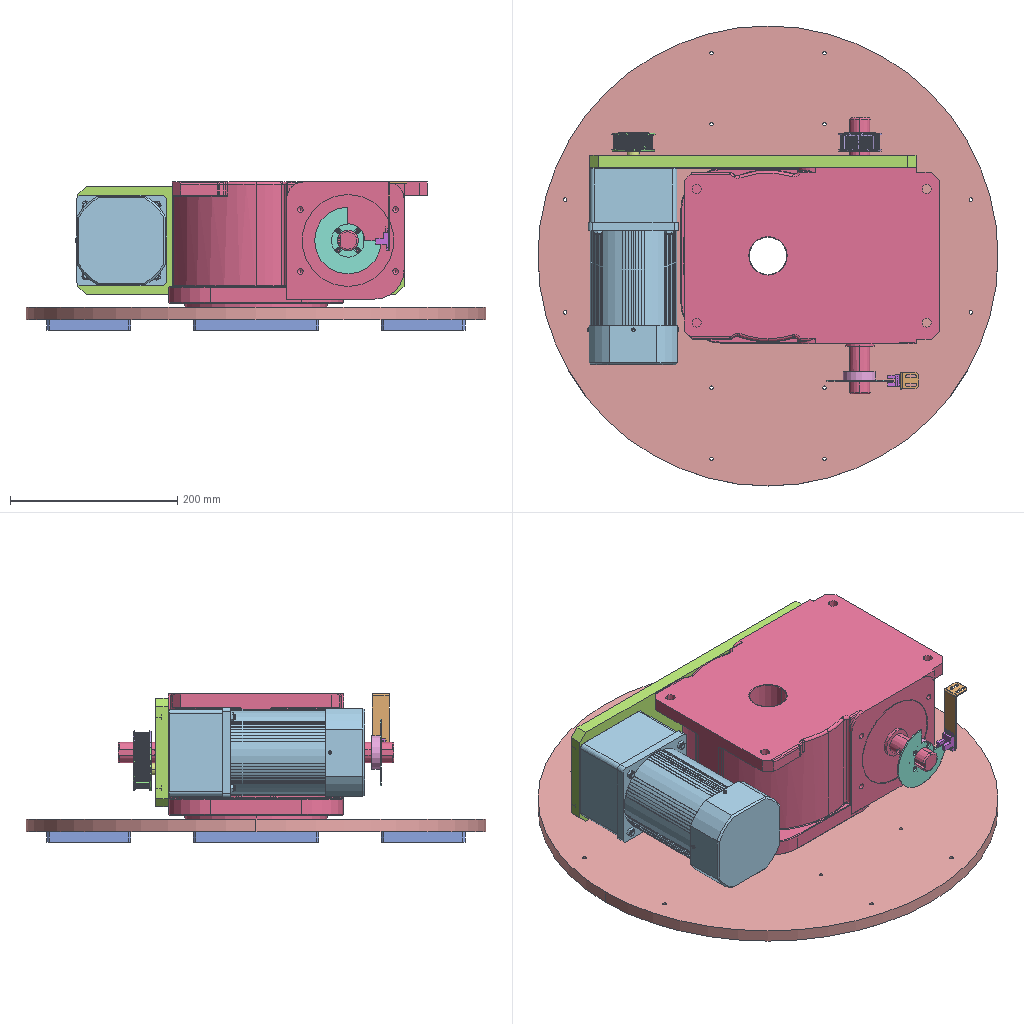Assembly | SolidWorks | 11 different items | 14 placed | box 550 x 550 x 177 mm
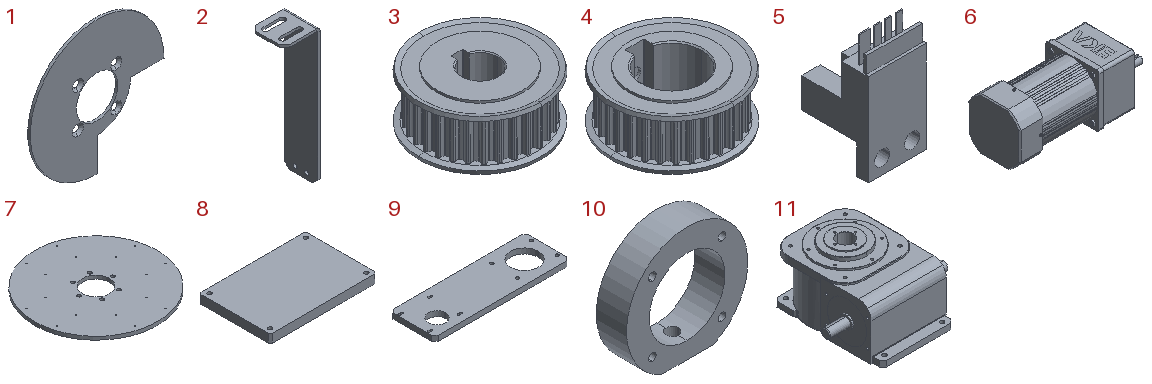Parts list (item | quantity | size | volume | features):
1 | x1 | 80 x 1.5 x 80 mm | 5264 mm3 | features FlatPattern 1, HoleWzd 1, SMBaseFlange 1, SheetMetal 1
2 | x1 | 21.5 x 20 x 81.5 mm | 2855 mm3 | features HoleWzd 2, Chamfer 1, FlatPattern 1, SMBaseFlange 1, SheetMetal 1
3 | x1 | 52 x 52 x 22 mm | 31133 mm3 | features BaseBody 1
4 | x1 | 52 x 52 x 22 mm | 23799 mm3 | features BaseBody 1
5 | x1 | 13.6 x 15.5 x 27.7 mm | 2033 mm3 | features BaseBody 1
6 | x1 | 277 x 108.652 x 108.652 mm | 2253105 mm3 | features BaseBody 2
7 | x1 | 550 x 550 x 15 mm | 3378940 mm3 | features CirPattern 2, HoleWzd 2, Cut 1, Extrusion 1
8 | x4 | 150 x 100 x 12 mm | 167862 mm3 | features Chamfer 1, Extrusion 1, HoleWzd 1, ICE 1
9 | x1 | 390 x 130 x 15 mm | 637753 mm3 | features HoleWzd 2, Chamfer 1, Cut 1, Extrusion 1
10 | x1 | 40 x 10 x 38 mm | 7150 mm3 | features HoleWzd 2, Extrusion 1, ICE 1
11 | x1 | 330 x 309.5 x 163 mm | 7808751 mm3 | features BaseBody 1
Mates (type | each side: item.copy, entity, surface, feature):
Concentric | 7.1 face cylinder Boss-Extrude1 | 11.1 face cylinder Imported1
Coincident | 7.1 face plane Boss-Extrude1 | 11.1 face plane Imported1
Coincident | 11.1 face plane Imported1 | assembly plane
Coincident | 7.1 plane | assembly plane | 2 times
Coincident | 7.1 face plane Boss-Extrude1 | 8.1 face plane Boss-Extrude1
Width | 8.1 face plane Boss-Extrude1 | 8.1 face plane Boss-Extrude1 | 7.1 face cylinder Boss-Extrude1
DistanceDim | 8.1 plane | assembly plane
Coincident | 8.1 plane | assembly plane
Coincident | 11.1 face plane Imported1 | 9.1 face plane Boss-Extrude1 | 2 times
Parallel | 11.1 face plane Imported1 | 7.1 plane
Parallel | 11.1 face plane Imported1 | 9.1 face plane Boss-Extrude1
Width | 11.1 face plane Imported1 | 11.1 face plane Imported1 | 9.1 face plane Boss-Extrude1 | 9.1 face plane Boss-Extrude1
Coincident | 9.1 face plane Boss-Extrude1 | 6.1 face plane Imported1 | 2 times
Width | 9.1 face plane Boss-Extrude1 | 9.1 face plane Boss-Extrude1 | 6.1 face plane Imported1 | 6.1 face plane Imported1
Concentric | 11.1 face cylinder Imported1 | 4.1 face cylinder Imported1
Coincident | 6.1 face plane Imported2 | 4.1 face plane Imported1
Concentric | 6.1 face cylinder Imported2 | 3.1 face cylinder Imported1
Coincident | 6.1 face plane Imported2 | 3.1 face plane Imported1
Concentric | 11.1 face cylinder Imported1 | 10.1 face cylinder Boss-Extrude1
Concentric | 10.1 face cylinder Boss-Extrude1 | 1.1 face cylinder Base-Flange1
Coincident | 10.1 face plane Boss-Extrude1 | 1.1 face plane Base-Flange1
DistanceDim | 1.1 face plane Base-Flange1 | 11.1 face plane Imported1
Coincident | 10.1 plane | 1.1 plane
Coincident | 11.1 face plane Imported1 | 2.1 face plane Base-Flange1
Width | 2.1 face plane Base-Flange1 | 2.1 face plane Base-Flange1 | 1.1 face plane Base-Flange1 | 1.1 face plane Base-Flange1
Coincident | 2.1 face plane Base-Flange1 | 5.1 face plane Imported1 | 2 times
Width | 2.1 face plane Base-Flange1 | 2.1 face plane Base-Flange1 | 5.1 face plane Imported1 | 5.1 face plane Imported1
DistanceDim | 2.1 face plane Base-Flange1 | 11.1 face plane Imported1
Parallel | 10.1 face plane Cut-Extrude1 | 11.1 face plane Imported1